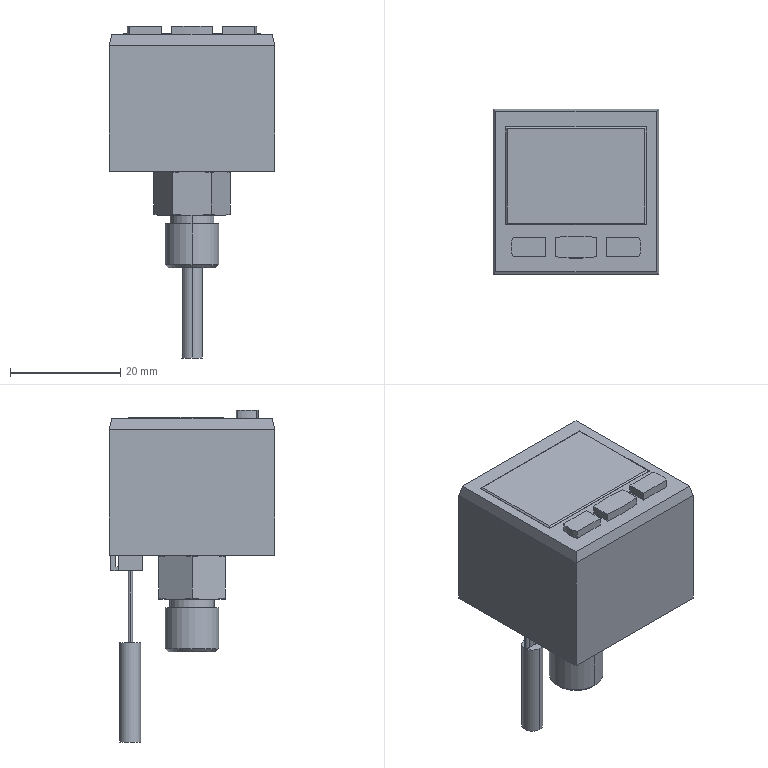Part | STEP file | ISE30A-01-N-ML_0_^气源二联件-SMC | 1 solid | 138 faces | box 30 x 30 x 60.1 mm | volume 24209 mm3 | plane 68 | cone 38 | cylinder 32 | commonest cylinder face diameters 0.88 x8 2.459 x4 2.6 x4 4 x4 3.8 x2 4.134 x2